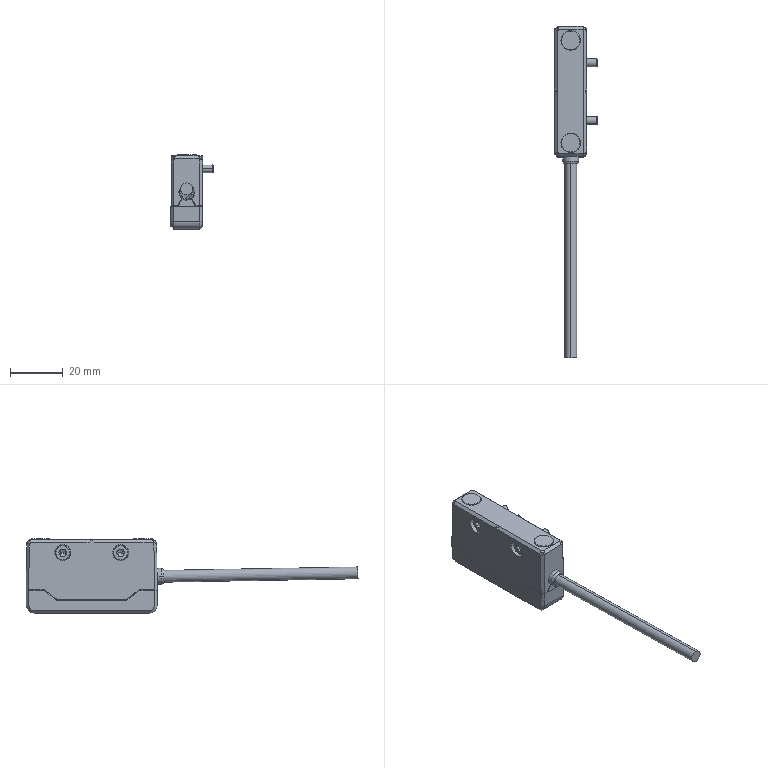Part | SolidWorks | features BaseBody 7 | 7 solids | 757 faces | box 16.008 x 126.481 x 28.318 mm | volume 9351 mm3 | plane 438 | spline 180 | cone 74 | cylinder 49 | torus 12 | sphere 4 | commonest cylinder face diameters 3.001 x12 0.4 x6 3 x4 3.084 x4 4.975 x4 5.5 x4